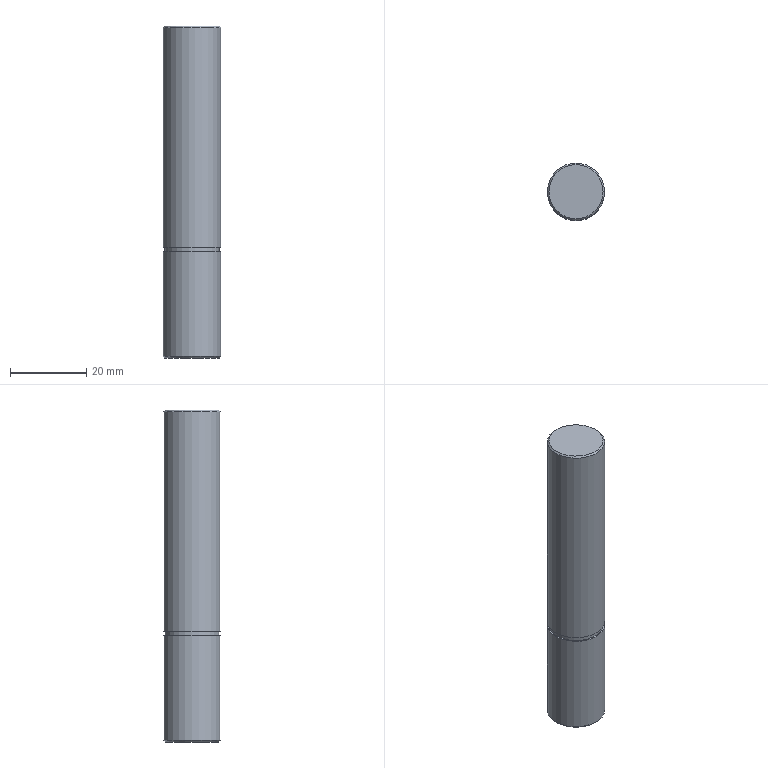Part | NX | features 5003_006_FPSFJFA-D15-L58.0-H29(Default) 2 | 1 solid | 9 faces | box 15 x 15 x 87 mm | volume 15348 mm3 | plane 4 | cylinder 3 | cone 2 | commonest cylinder face diameters 15 x2 14.3 x1
STEP:
#1=CARTESIAN_POINT('',(165.675,-322.,-257.15));
#2=VERTEX_POINT('',#1);
#3=CARTESIAN_POINT('',(158.525,-322.,-257.15));
#4=DIRECTION('',(0.,0.,1.));
#5=DIRECTION('',(1.,0.,0.));
#6=AXIS2_PLACEMENT_3D('',#3,#4,#5);
#7=CIRCLE('',#6,7.15);
#8=EDGE_CURVE('',#2,#2,#7,.T.);
#9=ORIENTED_EDGE('',*,*,#8,.T.);
#10=EDGE_LOOP('',(#9));
#11=FACE_BOUND('',#10,.T.);
#12=CARTESIAN_POINT('',(166.025,-322.,-257.15));
#13=VERTEX_POINT('',#12);
#14=CARTESIAN_POINT('',(158.525,-322.,-257.15));
#15=DIRECTION('',(0.,0.,1.));
#16=DIRECTION('',(1.,0.,0.));
#17=AXIS2_PLACEMENT_3D('',#14,#15,#16);
#18=CIRCLE('',#17,7.5);
#19=EDGE_CURVE('',#13,#13,#18,.F.);
#20=ORIENTED_EDGE('',*,*,#19,.T.);
#21=EDGE_LOOP('',(#20));
#22=FACE_BOUND('',#21,.T.);
#23=CARTESIAN_POINT('',(158.525,-322.,-257.15));
#24=DIRECTION('',(0.,0.,1.));
#25=DIRECTION('',(1.,0.,0.));
#26=AXIS2_PLACEMENT_3D('',#23,#24,#25);
#27=PLANE('',#26);
#28=ADVANCED_FACE('',(#11,#22),#27,.F.);
#29=CARTESIAN_POINT('',(151.025,-322.,-199.55));
#30=VERTEX_POINT('',#29);
#31=CARTESIAN_POINT('',(158.525,-322.,-199.55));
#32=DIRECTION('',(0.,0.,-1.));
#33=DIRECTION('',(-1.,0.,0.));
#34=AXIS2_PLACEMENT_3D('',#31,#32,#33);
#35=CIRCLE('',#34,7.5);
#36=EDGE_CURVE('',#30,#30,#35,.T.);
#37=ORIENTED_EDGE('',*,*,#36,.T.);
#38=EDGE_LOOP('',(#37));
#39=FACE_BOUND('',#38,.T.);
#40=ORIENTED_EDGE('',*,*,#19,.F.);
#41=EDGE_LOOP('',(#40));
#42=FACE_BOUND('',#41,.T.);
#43=CARTESIAN_POINT('',(158.525,-322.,-257.15));
#44=DIRECTION('',(0.,0.,-1.));
#45=DIRECTION('',(-1.,0.,0.));
#46=AXIS2_PLACEMENT_3D('',#43,#44,#45);
#47=CYLINDRICAL_SURFACE('',#46,7.5);
#48=ADVANCED_FACE('',(#39,#42),#47,.T.);
#49=CARTESIAN_POINT('',(151.425,-322.,-199.15));
#50=VERTEX_POINT('',#49);
#51=CARTESIAN_POINT('',(158.525,-322.,-199.15));
#52=DIRECTION('',(0.,0.,-1.));
#53=DIRECTION('',(-1.,0.,0.));
#54=AXIS2_PLACEMENT_3D('',#51,#52,#53);
#55=CIRCLE('',#54,7.1);
#56=EDGE_CURVE('',#50,#50,#55,.F.);
#57=ORIENTED_EDGE('',*,*,#56,.T.);
#58=EDGE_LOOP('',(#57));
#59=FACE_BOUND('',#58,.T.);
#60=CARTESIAN_POINT('',(158.525,-322.,-199.15));
#61=DIRECTION('',(0.,0.,-1.));
#62=DIRECTION('',(-1.,0.,0.));
#63=AXIS2_PLACEMENT_3D('',#60,#61,#62);
#64=PLANE('',#63);
#65=ADVANCED_FACE('',(#59),#64,.F.);
#66=ORIENTED_EDGE('',*,*,#56,.F.);
#67=EDGE_LOOP('',(#66));
#68=FACE_BOUND('',#67,.T.);
#69=ORIENTED_EDGE('',*,*,#36,.F.);
#70=EDGE_LOOP('',(#69));
#71=FACE_BOUND('',#70,.T.);
#72=CARTESIAN_POINT('',(158.525,-322.,-199.55));
#73=DIRECTION('',(0.,0.,-1.));
#74=DIRECTION('',(-1.,0.,0.));
#75=AXIS2_PLACEMENT_3D('',#72,#73,#74);
#76=CONICAL_SURFACE('',#75,7.5,0.7854);
#77=ADVANCED_FACE('',(#68,#71),#76,.T.);
#78=CARTESIAN_POINT('',(151.425,-322.,-286.15));
#79=VERTEX_POINT('',#78);
#80=CARTESIAN_POINT('',(158.525,-322.,-286.15));
#81=DIRECTION('',(0.,0.,-1.));
#82=DIRECTION('',(-1.,0.,0.));
#83=AXIS2_PLACEMENT_3D('',#80,#81,#82);
#84=CIRCLE('',#83,7.1);
#85=EDGE_CURVE('',#79,#79,#84,.T.);
#86=ORIENTED_EDGE('',*,*,#85,.T.);
#87=EDGE_LOOP('',(#86));
#88=FACE_BOUND('',#87,.T.);
#89=CARTESIAN_POINT('',(158.525,-314.5,-286.15));
#90=DIRECTION('',(0.,0.,-1.));
#91=DIRECTION('',(-1.,0.,0.));
#92=AXIS2_PLACEMENT_3D('',#89,#90,#91);
#93=PLANE('',#92);
#94=ADVANCED_FACE('',(#88),#93,.T.);
#95=CARTESIAN_POINT('',(165.675,-322.,-258.3));
#96=VERTEX_POINT('',#95);
#97=CARTESIAN_POINT('',(158.525,-322.,-258.3));
#98=DIRECTION('',(0.,0.,1.));
#99=DIRECTION('',(1.,0.,0.));
#100=AXIS2_PLACEMENT_3D('',#97,#98,#99);
#101=CIRCLE('',#100,7.15);
#102=EDGE_CURVE('',#96,#96,#101,.T.);
#103=ORIENTED_EDGE('',*,*,#102,.T.);
#104=EDGE_LOOP('',(#103));
#105=FACE_BOUND('',#104,.T.);
#106=ORIENTED_EDGE('',*,*,#8,.F.);
#107=EDGE_LOOP('',(#106));
#108=FACE_BOUND('',#107,.T.);
#109=CARTESIAN_POINT('',(158.525,-322.,-257.15));
#110=DIRECTION('',(0.,0.,1.));
#111=DIRECTION('',(1.,0.,0.));
#112=AXIS2_PLACEMENT_3D('',#109,#110,#111);
#113=CYLINDRICAL_SURFACE('',#112,7.15);
#114=ADVANCED_FACE('',(#105,#108),#113,.T.);
#115=CARTESIAN_POINT('',(166.025,-322.,-258.3));
#116=VERTEX_POINT('',#115);
#117=CARTESIAN_POINT('',(158.525,-322.,-258.3));
#118=DIRECTION('',(0.,0.,1.));
#119=DIRECTION('',(1.,0.,0.));
#120=AXIS2_PLACEMENT_3D('',#117,#118,#119);
#121=CIRCLE('',#120,7.5);
#122=EDGE_CURVE('',#116,#116,#121,.T.);
#123=ORIENTED_EDGE('',*,*,#122,.T.);
#124=EDGE_LOOP('',(#123));
#125=FACE_BOUND('',#124,.T.);
#126=ORIENTED_EDGE('',*,*,#102,.F.);
#127=EDGE_LOOP('',(#126));
#128=FACE_BOUND('',#127,.T.);
#129=CARTESIAN_POINT('',(158.525,-314.5,-258.3));
#130=DIRECTION('',(0.,0.,1.));
#131=DIRECTION('',(1.,0.,0.));
#132=AXIS2_PLACEMENT_3D('',#129,#130,#131);
#133=PLANE('',#132);
#134=ADVANCED_FACE('',(#125,#128),#133,.T.);
#135=CARTESIAN_POINT('',(151.025,-322.,-285.75));
#136=VERTEX_POINT('',#135);
#137=CARTESIAN_POINT('',(158.525,-322.,-285.75));
#138=DIRECTION('',(0.,0.,-1.));
#139=DIRECTION('',(-1.,0.,0.));
#140=AXIS2_PLACEMENT_3D('',#137,#138,#139);
#141=CIRCLE('',#140,7.5);
#142=EDGE_CURVE('',#136,#136,#141,.F.);
#143=ORIENTED_EDGE('',*,*,#142,.T.);
#144=EDGE_LOOP('',(#143));
#145=FACE_BOUND('',#144,.T.);
#146=ORIENTED_EDGE('',*,*,#122,.F.);
#147=EDGE_LOOP('',(#146));
#148=FACE_BOUND('',#147,.T.);
#149=CARTESIAN_POINT('',(158.525,-322.,-257.15));
#150=DIRECTION('',(0.,0.,1.));
#151=DIRECTION('',(1.,0.,0.));
#152=AXIS2_PLACEMENT_3D('',#149,#150,#151);
#153=CYLINDRICAL_SURFACE('',#152,7.5);
#154=ADVANCED_FACE('',(#145,#148),#153,.T.);
#155=ORIENTED_EDGE('',*,*,#85,.F.);
#156=EDGE_LOOP('',(#155));
#157=FACE_BOUND('',#156,.T.);
#158=ORIENTED_EDGE('',*,*,#142,.F.);
#159=EDGE_LOOP('',(#158));
#160=FACE_BOUND('',#159,.T.);
#161=CARTESIAN_POINT('',(158.525,-322.,-285.75));
#162=DIRECTION('',(0.,0.,1.));
#163=DIRECTION('',(1.,0.,0.));
#164=AXIS2_PLACEMENT_3D('',#161,#162,#163);
#165=CONICAL_SURFACE('',#164,7.5,0.7854);
#166=ADVANCED_FACE('',(#157,#160),#165,.T.);
#167=CLOSED_SHELL('',(#28,#48,#65,#77,#94,#114,#134,#154,#166));
#168=MANIFOLD_SOLID_BREP('',#167);
#169=(LENGTH_UNIT()NAMED_UNIT(*)SI_UNIT(.MILLI.,.METRE.));
#170=UNCERTAINTY_MEASURE_WITH_UNIT(LENGTH_MEASURE(0.00001),#169,'','');
#171=(NAMED_UNIT(*)PLANE_ANGLE_UNIT()SI_UNIT($,.RADIAN.));
#172=(NAMED_UNIT(*)SI_UNIT($,.STERADIAN.)SOLID_ANGLE_UNIT());
#173=(GEOMETRIC_REPRESENTATION_CONTEXT(3)GLOBAL_UNCERTAINTY_ASSIGNED_CONTEXT((#170))GLOBAL_UNIT_ASSIGNED_CONTEXT((#169,#171,#172))REPRESENTATION_CONTEXT('',''));
#174=ADVANCED_BREP_SHAPE_REPRESENTATION('',(#168),#173);